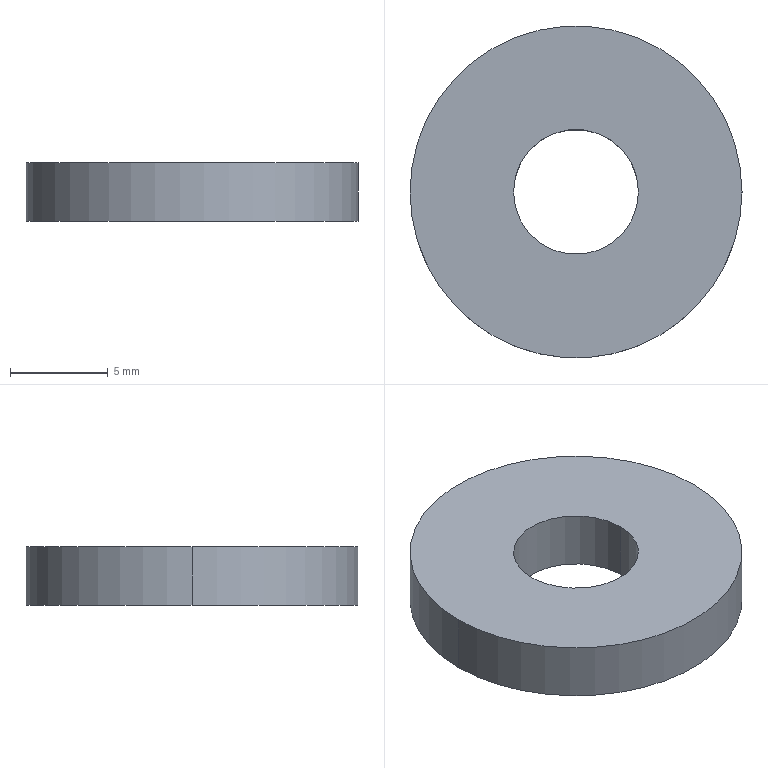Part | NX | features BREP 1 | 1 solid | 6 faces | box 17 x 17 x 3 mm | volume 584.43 mm3 | cylinder 4 | plane 2 | commonest cylinder face diameters 6.4 x2 17 x2
STEP:
#1=CARTESIAN_POINT('',(-3.2,0.,3.));
#2=VERTEX_POINT('',#1);
#3=CARTESIAN_POINT('',(3.2,0.,3.));
#4=VERTEX_POINT('',#3);
#5=CARTESIAN_POINT('',(0.,0.,3.));
#6=DIRECTION('',(0.,0.,1.));
#7=DIRECTION('',(1.,0.,0.));
#8=AXIS2_PLACEMENT_3D('',#5,#6,#7);
#9=CIRCLE('',#8,3.2);
#10=EDGE_CURVE('',#2,#4,#9,.T.);
#11=ORIENTED_EDGE('',*,*,#10,.T.);
#12=CARTESIAN_POINT('',(3.2,0.,0.));
#13=VERTEX_POINT('',#12);
#14=CARTESIAN_POINT('',(3.2,0.,3.));
#15=DIRECTION('',(0.,0.,-1.));
#16=VECTOR('',#15,1000.);
#17=LINE('',#14,#16);
#18=EDGE_CURVE('',#13,#4,#17,.F.);
#19=ORIENTED_EDGE('',*,*,#18,.F.);
#20=CARTESIAN_POINT('',(-3.2,0.,0.));
#21=VERTEX_POINT('',#20);
#22=CARTESIAN_POINT('',(0.,0.,0.));
#23=DIRECTION('',(0.,0.,1.));
#24=DIRECTION('',(1.,0.,0.));
#25=AXIS2_PLACEMENT_3D('',#22,#23,#24);
#26=CIRCLE('',#25,3.2);
#27=EDGE_CURVE('',#21,#13,#26,.T.);
#28=ORIENTED_EDGE('',*,*,#27,.F.);
#29=CARTESIAN_POINT('',(-3.2,0.,3.));
#30=DIRECTION('',(0.,0.,-1.));
#31=VECTOR('',#30,1000.);
#32=LINE('',#29,#31);
#33=EDGE_CURVE('',#21,#2,#32,.F.);
#34=ORIENTED_EDGE('',*,*,#33,.T.);
#35=EDGE_LOOP('',(#11,#19,#28,#34));
#36=FACE_BOUND('',#35,.T.);
#37=CARTESIAN_POINT('',(0.,0.,3.));
#38=DIRECTION('',(0.,0.,-1.));
#39=DIRECTION('',(1.,0.,0.));
#40=AXIS2_PLACEMENT_3D('',#37,#38,#39);
#41=CYLINDRICAL_SURFACE('',#40,3.2);
#42=ADVANCED_FACE('',(#36),#41,.F.);
#43=CARTESIAN_POINT('',(8.5,0.,3.));
#44=VERTEX_POINT('',#43);
#45=CARTESIAN_POINT('',(-8.5,0.,3.));
#46=VERTEX_POINT('',#45);
#47=CARTESIAN_POINT('',(0.,0.,3.));
#48=DIRECTION('',(0.,0.,1.));
#49=DIRECTION('',(1.,0.,0.));
#50=AXIS2_PLACEMENT_3D('',#47,#48,#49);
#51=CIRCLE('',#50,8.5);
#52=EDGE_CURVE('',#44,#46,#51,.T.);
#53=ORIENTED_EDGE('',*,*,#52,.F.);
#54=CARTESIAN_POINT('',(8.5,0.,0.));
#55=VERTEX_POINT('',#54);
#56=CARTESIAN_POINT('',(8.5,0.,3.));
#57=DIRECTION('',(0.,0.,-1.));
#58=VECTOR('',#57,1000.);
#59=LINE('',#56,#58);
#60=EDGE_CURVE('',#55,#44,#59,.F.);
#61=ORIENTED_EDGE('',*,*,#60,.F.);
#62=CARTESIAN_POINT('',(-8.5,0.,0.));
#63=VERTEX_POINT('',#62);
#64=CARTESIAN_POINT('',(0.,0.,0.));
#65=DIRECTION('',(0.,0.,1.));
#66=DIRECTION('',(1.,0.,0.));
#67=AXIS2_PLACEMENT_3D('',#64,#65,#66);
#68=CIRCLE('',#67,8.5);
#69=EDGE_CURVE('',#55,#63,#68,.T.);
#70=ORIENTED_EDGE('',*,*,#69,.T.);
#71=CARTESIAN_POINT('',(-8.5,0.,3.));
#72=DIRECTION('',(0.,0.,-1.));
#73=VECTOR('',#72,1000.);
#74=LINE('',#71,#73);
#75=EDGE_CURVE('',#63,#46,#74,.F.);
#76=ORIENTED_EDGE('',*,*,#75,.T.);
#77=EDGE_LOOP('',(#53,#61,#70,#76));
#78=FACE_BOUND('',#77,.T.);
#79=CARTESIAN_POINT('',(0.,0.,3.));
#80=DIRECTION('',(0.,0.,-1.));
#81=DIRECTION('',(1.,0.,0.));
#82=AXIS2_PLACEMENT_3D('',#79,#80,#81);
#83=CYLINDRICAL_SURFACE('',#82,8.5);
#84=ADVANCED_FACE('',(#78),#83,.T.);
#85=CARTESIAN_POINT('',(0.,0.,3.));
#86=DIRECTION('',(0.,0.,1.));
#87=DIRECTION('',(1.,0.,0.));
#88=AXIS2_PLACEMENT_3D('',#85,#86,#87);
#89=CIRCLE('',#88,8.5);
#90=EDGE_CURVE('',#46,#44,#89,.T.);
#91=ORIENTED_EDGE('',*,*,#90,.T.);
#92=ORIENTED_EDGE('',*,*,#52,.T.);
#93=EDGE_LOOP('',(#91,#92));
#94=FACE_BOUND('',#93,.T.);
#95=ORIENTED_EDGE('',*,*,#10,.F.);
#96=CARTESIAN_POINT('',(0.,0.,3.));
#97=DIRECTION('',(0.,0.,1.));
#98=DIRECTION('',(1.,0.,0.));
#99=AXIS2_PLACEMENT_3D('',#96,#97,#98);
#100=CIRCLE('',#99,3.2);
#101=EDGE_CURVE('',#4,#2,#100,.T.);
#102=ORIENTED_EDGE('',*,*,#101,.F.);
#103=EDGE_LOOP('',(#95,#102));
#104=FACE_BOUND('',#103,.T.);
#105=CARTESIAN_POINT('',(0.,0.,3.));
#106=DIRECTION('',(0.,0.,1.));
#107=DIRECTION('',(-1.,0.,0.));
#108=AXIS2_PLACEMENT_3D('',#105,#106,#107);
#109=PLANE('',#108);
#110=ADVANCED_FACE('',(#94,#104),#109,.T.);
#111=CARTESIAN_POINT('',(0.,0.,0.));
#112=DIRECTION('',(0.,0.,1.));
#113=DIRECTION('',(1.,0.,0.));
#114=AXIS2_PLACEMENT_3D('',#111,#112,#113);
#115=CIRCLE('',#114,8.5);
#116=EDGE_CURVE('',#63,#55,#115,.T.);
#117=ORIENTED_EDGE('',*,*,#116,.F.);
#118=ORIENTED_EDGE('',*,*,#69,.F.);
#119=EDGE_LOOP('',(#117,#118));
#120=FACE_BOUND('',#119,.T.);
#121=ORIENTED_EDGE('',*,*,#27,.T.);
#122=CARTESIAN_POINT('',(0.,0.,0.));
#123=DIRECTION('',(0.,0.,1.));
#124=DIRECTION('',(1.,0.,0.));
#125=AXIS2_PLACEMENT_3D('',#122,#123,#124);
#126=CIRCLE('',#125,3.2);
#127=EDGE_CURVE('',#13,#21,#126,.T.);
#128=ORIENTED_EDGE('',*,*,#127,.T.);
#129=EDGE_LOOP('',(#121,#128));
#130=FACE_BOUND('',#129,.T.);
#131=CARTESIAN_POINT('',(0.,0.,0.));
#132=DIRECTION('',(0.,0.,1.));
#133=DIRECTION('',(-1.,0.,0.));
#134=AXIS2_PLACEMENT_3D('',#131,#132,#133);
#135=PLANE('',#134);
#136=ADVANCED_FACE('',(#120,#130),#135,.F.);
#137=ORIENTED_EDGE('',*,*,#60,.T.);
#138=ORIENTED_EDGE('',*,*,#90,.F.);
#139=ORIENTED_EDGE('',*,*,#75,.F.);
#140=ORIENTED_EDGE('',*,*,#116,.T.);
#141=EDGE_LOOP('',(#137,#138,#139,#140));
#142=FACE_BOUND('',#141,.T.);
#143=CARTESIAN_POINT('',(0.,0.,3.));
#144=DIRECTION('',(0.,0.,-1.));
#145=DIRECTION('',(1.,0.,0.));
#146=AXIS2_PLACEMENT_3D('',#143,#144,#145);
#147=CYLINDRICAL_SURFACE('',#146,8.5);
#148=ADVANCED_FACE('',(#142),#147,.T.);
#149=ORIENTED_EDGE('',*,*,#18,.T.);
#150=ORIENTED_EDGE('',*,*,#101,.T.);
#151=ORIENTED_EDGE('',*,*,#33,.F.);
#152=ORIENTED_EDGE('',*,*,#127,.F.);
#153=EDGE_LOOP('',(#149,#150,#151,#152));
#154=FACE_BOUND('',#153,.T.);
#155=CARTESIAN_POINT('',(0.,0.,3.));
#156=DIRECTION('',(0.,0.,-1.));
#157=DIRECTION('',(1.,0.,0.));
#158=AXIS2_PLACEMENT_3D('',#155,#156,#157);
#159=CYLINDRICAL_SURFACE('',#158,3.2);
#160=ADVANCED_FACE('',(#154),#159,.F.);
#161=CLOSED_SHELL('',(#42,#84,#110,#136,#148,#160));
#162=MANIFOLD_SOLID_BREP('',#161);
#163=(LENGTH_UNIT()NAMED_UNIT(*)SI_UNIT(.MILLI.,.METRE.));
#164=UNCERTAINTY_MEASURE_WITH_UNIT(LENGTH_MEASURE(0.00001),#163,'','');
#165=(NAMED_UNIT(*)PLANE_ANGLE_UNIT()SI_UNIT($,.RADIAN.));
#166=(NAMED_UNIT(*)SI_UNIT($,.STERADIAN.)SOLID_ANGLE_UNIT());
#167=(GEOMETRIC_REPRESENTATION_CONTEXT(3)GLOBAL_UNCERTAINTY_ASSIGNED_CONTEXT((#164))GLOBAL_UNIT_ASSIGNED_CONTEXT((#163,#165,#166))REPRESENTATION_CONTEXT('',''));
#168=ADVANCED_BREP_SHAPE_REPRESENTATION('',(#162),#167);